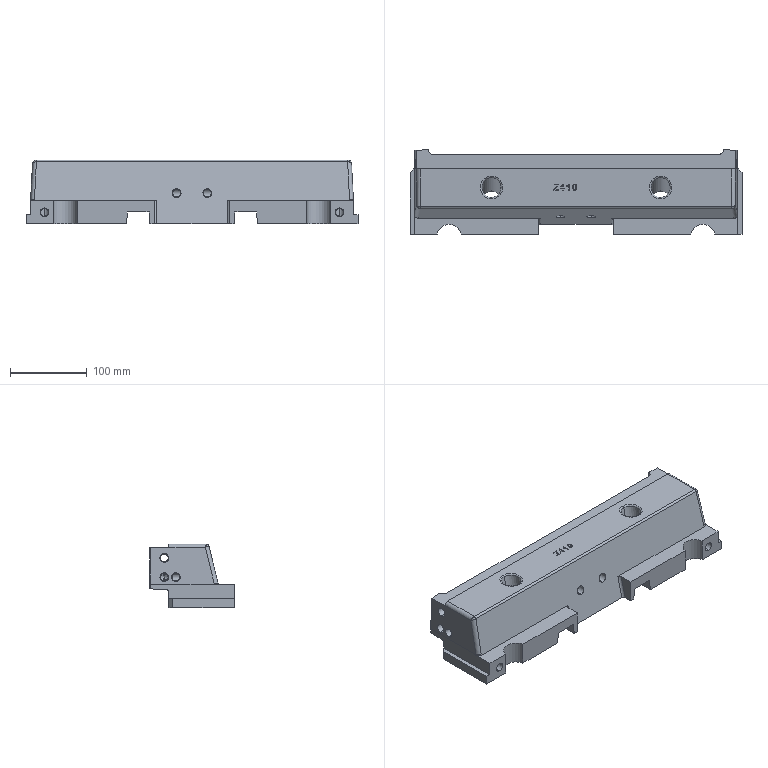Part | Creo | 1 solid | 216 faces | box 432 x 109.954 x 83 mm | volume 2427857 mm3 | plane 97 | cylinder 97 | spline 8 | other 8 | cone 4 | torus 2 | commonest cylinder face diameters 10 x44 11.4 x28 16 x6 6 x4 12 x4 25 x4